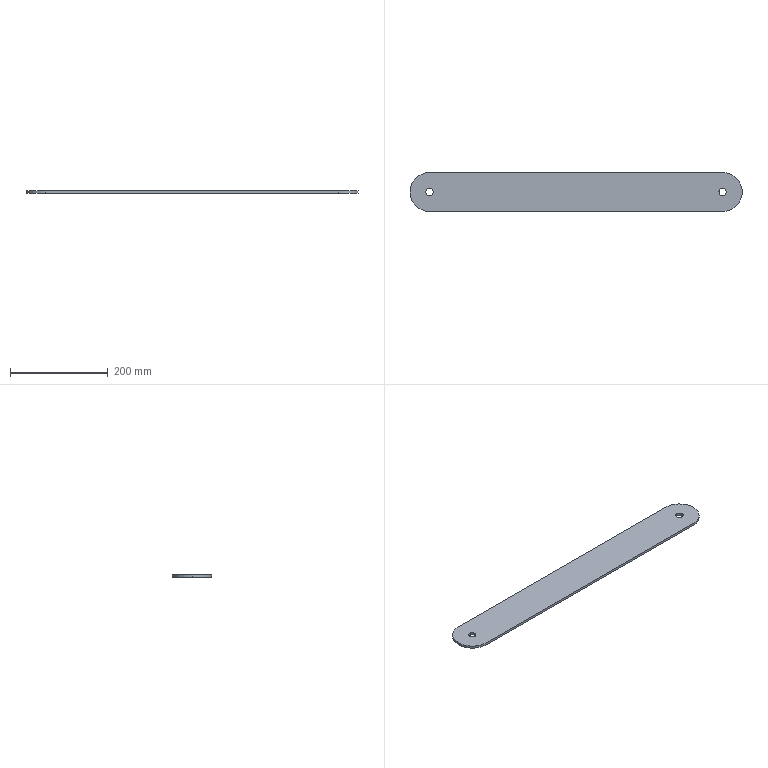Part | SolidWorks | features Extrusion 1, ICE 1 | 1 solid | 11 faces | box 680 x 80 x 5 mm | volume 263366 mm3 | cylinder 7 | plane 4 | commonest cylinder face diameters 15 x4 80 x3
STEP:
#1=CARTESIAN_POINT('',(-7.5,0.,0.));
#2=VERTEX_POINT('',#1);
#3=CARTESIAN_POINT('',(7.5,0.,0.));
#4=VERTEX_POINT('',#3);
#5=CARTESIAN_POINT('',(0.,0.,0.));
#6=DIRECTION('',(0.,0.,1.));
#7=DIRECTION('',(1.,0.,0.));
#8=AXIS2_PLACEMENT_3D('',#5,#6,#7);
#9=CIRCLE('',#8,7.5);
#10=EDGE_CURVE('',#2,#4,#9,.T.);
#11=ORIENTED_EDGE('',*,*,#10,.F.);
#12=CARTESIAN_POINT('',(-7.5,0.,5.));
#13=VERTEX_POINT('',#12);
#14=CARTESIAN_POINT('',(-7.5,0.,0.));
#15=DIRECTION('',(0.,0.,1.));
#16=VECTOR('',#15,1000.);
#17=LINE('',#14,#16);
#18=EDGE_CURVE('',#2,#13,#17,.T.);
#19=ORIENTED_EDGE('',*,*,#18,.T.);
#20=CARTESIAN_POINT('',(7.5,0.,5.));
#21=VERTEX_POINT('',#20);
#22=CARTESIAN_POINT('',(0.,0.,5.));
#23=DIRECTION('',(0.,0.,1.));
#24=DIRECTION('',(1.,0.,0.));
#25=AXIS2_PLACEMENT_3D('',#22,#23,#24);
#26=CIRCLE('',#25,7.5);
#27=EDGE_CURVE('',#13,#21,#26,.T.);
#28=ORIENTED_EDGE('',*,*,#27,.T.);
#29=CARTESIAN_POINT('',(7.5,0.,0.));
#30=DIRECTION('',(0.,0.,1.));
#31=VECTOR('',#30,1000.);
#32=LINE('',#29,#31);
#33=EDGE_CURVE('',#4,#21,#32,.T.);
#34=ORIENTED_EDGE('',*,*,#33,.F.);
#35=EDGE_LOOP('',(#11,#19,#28,#34));
#36=FACE_OUTER_BOUND('',#35,.T.);
#37=CARTESIAN_POINT('',(0.,0.,0.));
#38=DIRECTION('',(0.,0.,1.));
#39=DIRECTION('',(1.,0.,0.));
#40=AXIS2_PLACEMENT_3D('',#37,#38,#39);
#41=CYLINDRICAL_SURFACE('',#40,7.5);
#42=ADVANCED_FACE('',(#36),#41,.F.);
#43=CARTESIAN_POINT('',(592.5,0.,0.));
#44=VERTEX_POINT('',#43);
#45=CARTESIAN_POINT('',(607.5,0.,0.));
#46=VERTEX_POINT('',#45);
#47=CARTESIAN_POINT('',(600.,0.,0.));
#48=DIRECTION('',(0.,0.,1.));
#49=DIRECTION('',(1.,0.,0.));
#50=AXIS2_PLACEMENT_3D('',#47,#48,#49);
#51=CIRCLE('',#50,7.5);
#52=EDGE_CURVE('',#44,#46,#51,.T.);
#53=ORIENTED_EDGE('',*,*,#52,.F.);
#54=CARTESIAN_POINT('',(592.5,0.,5.));
#55=VERTEX_POINT('',#54);
#56=CARTESIAN_POINT('',(592.5,0.,0.));
#57=DIRECTION('',(0.,0.,1.));
#58=VECTOR('',#57,1000.);
#59=LINE('',#56,#58);
#60=EDGE_CURVE('',#44,#55,#59,.T.);
#61=ORIENTED_EDGE('',*,*,#60,.T.);
#62=CARTESIAN_POINT('',(607.5,0.,5.));
#63=VERTEX_POINT('',#62);
#64=CARTESIAN_POINT('',(600.,0.,5.));
#65=DIRECTION('',(0.,0.,1.));
#66=DIRECTION('',(1.,0.,0.));
#67=AXIS2_PLACEMENT_3D('',#64,#65,#66);
#68=CIRCLE('',#67,7.5);
#69=EDGE_CURVE('',#55,#63,#68,.T.);
#70=ORIENTED_EDGE('',*,*,#69,.T.);
#71=CARTESIAN_POINT('',(607.5,0.,0.));
#72=DIRECTION('',(0.,0.,1.));
#73=VECTOR('',#72,1000.);
#74=LINE('',#71,#73);
#75=EDGE_CURVE('',#46,#63,#74,.T.);
#76=ORIENTED_EDGE('',*,*,#75,.F.);
#77=EDGE_LOOP('',(#53,#61,#70,#76));
#78=FACE_OUTER_BOUND('',#77,.T.);
#79=CARTESIAN_POINT('',(600.,0.,0.));
#80=DIRECTION('',(0.,0.,1.));
#81=DIRECTION('',(1.,0.,0.));
#82=AXIS2_PLACEMENT_3D('',#79,#80,#81);
#83=CYLINDRICAL_SURFACE('',#82,7.5);
#84=ADVANCED_FACE('',(#78),#83,.F.);
#85=CARTESIAN_POINT('',(-40.,0.,5.));
#86=VERTEX_POINT('',#85);
#87=CARTESIAN_POINT('',(0.,-40.,5.));
#88=VERTEX_POINT('',#87);
#89=CARTESIAN_POINT('',(0.,0.,5.));
#90=DIRECTION('',(0.,0.,1.));
#91=DIRECTION('',(1.,0.,0.));
#92=AXIS2_PLACEMENT_3D('',#89,#90,#91);
#93=CIRCLE('',#92,40.);
#94=EDGE_CURVE('',#86,#88,#93,.T.);
#95=ORIENTED_EDGE('',*,*,#94,.F.);
#96=CARTESIAN_POINT('',(-40.,0.,0.));
#97=VERTEX_POINT('',#96);
#98=CARTESIAN_POINT('',(-40.,0.,5.));
#99=DIRECTION('',(0.,0.,-1.));
#100=VECTOR('',#99,1000.);
#101=LINE('',#98,#100);
#102=EDGE_CURVE('',#86,#97,#101,.T.);
#103=ORIENTED_EDGE('',*,*,#102,.T.);
#104=CARTESIAN_POINT('',(0.,-40.,0.));
#105=VERTEX_POINT('',#104);
#106=CARTESIAN_POINT('',(0.,0.,0.));
#107=DIRECTION('',(0.,0.,1.));
#108=DIRECTION('',(1.,0.,0.));
#109=AXIS2_PLACEMENT_3D('',#106,#107,#108);
#110=CIRCLE('',#109,40.);
#111=EDGE_CURVE('',#97,#105,#110,.T.);
#112=ORIENTED_EDGE('',*,*,#111,.T.);
#113=CARTESIAN_POINT('',(0.,-40.,5.));
#114=DIRECTION('',(0.,0.,-1.));
#115=VECTOR('',#114,1000.);
#116=LINE('',#113,#115);
#117=EDGE_CURVE('',#88,#105,#116,.T.);
#118=ORIENTED_EDGE('',*,*,#117,.F.);
#119=EDGE_LOOP('',(#95,#103,#112,#118));
#120=FACE_OUTER_BOUND('',#119,.T.);
#121=CARTESIAN_POINT('',(0.,0.,5.));
#122=DIRECTION('',(0.,0.,-1.));
#123=DIRECTION('',(-1.,0.,0.));
#124=AXIS2_PLACEMENT_3D('',#121,#122,#123);
#125=CYLINDRICAL_SURFACE('',#124,40.);
#126=ADVANCED_FACE('',(#120),#125,.T.);
#127=ORIENTED_EDGE('',*,*,#102,.F.);
#128=CARTESIAN_POINT('',(0.,40.,5.));
#129=VERTEX_POINT('',#128);
#130=CARTESIAN_POINT('',(0.,0.,5.));
#131=DIRECTION('',(0.,0.,1.));
#132=DIRECTION('',(1.,0.,0.));
#133=AXIS2_PLACEMENT_3D('',#130,#131,#132);
#134=CIRCLE('',#133,40.);
#135=EDGE_CURVE('',#129,#86,#134,.T.);
#136=ORIENTED_EDGE('',*,*,#135,.F.);
#137=CARTESIAN_POINT('',(0.,40.,0.));
#138=VERTEX_POINT('',#137);
#139=CARTESIAN_POINT('',(0.,40.,5.));
#140=DIRECTION('',(0.,0.,-1.));
#141=VECTOR('',#140,1000.);
#142=LINE('',#139,#141);
#143=EDGE_CURVE('',#129,#138,#142,.T.);
#144=ORIENTED_EDGE('',*,*,#143,.T.);
#145=CARTESIAN_POINT('',(0.,0.,0.));
#146=DIRECTION('',(0.,0.,1.));
#147=DIRECTION('',(1.,0.,0.));
#148=AXIS2_PLACEMENT_3D('',#145,#146,#147);
#149=CIRCLE('',#148,40.);
#150=EDGE_CURVE('',#138,#97,#149,.T.);
#151=ORIENTED_EDGE('',*,*,#150,.T.);
#152=EDGE_LOOP('',(#127,#136,#144,#151));
#153=FACE_OUTER_BOUND('',#152,.T.);
#154=CARTESIAN_POINT('',(0.,0.,5.));
#155=DIRECTION('',(0.,0.,-1.));
#156=DIRECTION('',(-1.,0.,0.));
#157=AXIS2_PLACEMENT_3D('',#154,#155,#156);
#158=CYLINDRICAL_SURFACE('',#157,40.);
#159=ADVANCED_FACE('',(#153),#158,.T.);
#160=CARTESIAN_POINT('',(600.,-40.,0.));
#161=VERTEX_POINT('',#160);
#162=CARTESIAN_POINT('',(0.,-40.,0.));
#163=DIRECTION('',(1.,0.,0.));
#164=VECTOR('',#163,1000.);
#165=LINE('',#162,#164);
#166=EDGE_CURVE('',#105,#161,#165,.T.);
#167=ORIENTED_EDGE('',*,*,#166,.T.);
#168=CARTESIAN_POINT('',(600.,-40.,5.));
#169=VERTEX_POINT('',#168);
#170=CARTESIAN_POINT('',(600.,-40.,5.));
#171=DIRECTION('',(0.,0.,-1.));
#172=VECTOR('',#171,1000.);
#173=LINE('',#170,#172);
#174=EDGE_CURVE('',#169,#161,#173,.T.);
#175=ORIENTED_EDGE('',*,*,#174,.F.);
#176=CARTESIAN_POINT('',(0.,-40.,5.));
#177=DIRECTION('',(1.,0.,0.));
#178=VECTOR('',#177,1000.);
#179=LINE('',#176,#178);
#180=EDGE_CURVE('',#88,#169,#179,.T.);
#181=ORIENTED_EDGE('',*,*,#180,.F.);
#182=ORIENTED_EDGE('',*,*,#117,.T.);
#183=EDGE_LOOP('',(#167,#175,#181,#182));
#184=FACE_OUTER_BOUND('',#183,.T.);
#185=CARTESIAN_POINT('',(0.,-40.,5.));
#186=DIRECTION('',(0.,1.,0.));
#187=DIRECTION('',(0.,0.,1.));
#188=AXIS2_PLACEMENT_3D('',#185,#186,#187);
#189=PLANE('',#188);
#190=ADVANCED_FACE('',(#184),#189,.F.);
#191=CARTESIAN_POINT('',(600.,40.,0.));
#192=VERTEX_POINT('',#191);
#193=CARTESIAN_POINT('',(600.,0.,0.));
#194=DIRECTION('',(0.,0.,1.));
#195=DIRECTION('',(1.,0.,0.));
#196=AXIS2_PLACEMENT_3D('',#193,#194,#195);
#197=CIRCLE('',#196,40.);
#198=EDGE_CURVE('',#161,#192,#197,.T.);
#199=ORIENTED_EDGE('',*,*,#198,.T.);
#200=CARTESIAN_POINT('',(600.,40.,5.));
#201=VERTEX_POINT('',#200);
#202=CARTESIAN_POINT('',(600.,40.,5.));
#203=DIRECTION('',(0.,0.,-1.));
#204=VECTOR('',#203,1000.);
#205=LINE('',#202,#204);
#206=EDGE_CURVE('',#201,#192,#205,.T.);
#207=ORIENTED_EDGE('',*,*,#206,.F.);
#208=CARTESIAN_POINT('',(600.,0.,5.));
#209=DIRECTION('',(0.,0.,1.));
#210=DIRECTION('',(1.,0.,0.));
#211=AXIS2_PLACEMENT_3D('',#208,#209,#210);
#212=CIRCLE('',#211,40.);
#213=EDGE_CURVE('',#169,#201,#212,.T.);
#214=ORIENTED_EDGE('',*,*,#213,.F.);
#215=ORIENTED_EDGE('',*,*,#174,.T.);
#216=EDGE_LOOP('',(#199,#207,#214,#215));
#217=FACE_OUTER_BOUND('',#216,.T.);
#218=CARTESIAN_POINT('',(600.,0.,5.));
#219=DIRECTION('',(0.,0.,-1.));
#220=DIRECTION('',(-1.,0.,0.));
#221=AXIS2_PLACEMENT_3D('',#218,#219,#220);
#222=CYLINDRICAL_SURFACE('',#221,40.);
#223=ADVANCED_FACE('',(#217),#222,.T.);
#224=CARTESIAN_POINT('',(0.,40.,0.));
#225=DIRECTION('',(-1.,0.,0.));
#226=VECTOR('',#225,1000.);
#227=LINE('',#224,#226);
#228=EDGE_CURVE('',#192,#138,#227,.T.);
#229=ORIENTED_EDGE('',*,*,#228,.T.);
#230=ORIENTED_EDGE('',*,*,#143,.F.);
#231=CARTESIAN_POINT('',(0.,40.,5.));
#232=DIRECTION('',(-1.,0.,0.));
#233=VECTOR('',#232,1000.);
#234=LINE('',#231,#233);
#235=EDGE_CURVE('',#201,#129,#234,.T.);
#236=ORIENTED_EDGE('',*,*,#235,.F.);
#237=ORIENTED_EDGE('',*,*,#206,.T.);
#238=EDGE_LOOP('',(#229,#230,#236,#237));
#239=FACE_OUTER_BOUND('',#238,.T.);
#240=CARTESIAN_POINT('',(0.,40.,5.));
#241=DIRECTION('',(0.,-1.,0.));
#242=DIRECTION('',(0.,0.,-1.));
#243=AXIS2_PLACEMENT_3D('',#240,#241,#242);
#244=PLANE('',#243);
#245=ADVANCED_FACE('',(#239),#244,.F.);
#246=CARTESIAN_POINT('',(0.,0.,5.));
#247=DIRECTION('',(0.,0.,1.));
#248=DIRECTION('',(1.,0.,0.));
#249=AXIS2_PLACEMENT_3D('',#246,#247,#248);
#250=CIRCLE('',#249,7.5);
#251=EDGE_CURVE('',#21,#13,#250,.T.);
#252=ORIENTED_EDGE('',*,*,#251,.F.);
#253=ORIENTED_EDGE('',*,*,#27,.F.);
#254=EDGE_LOOP('',(#252,#253));
#255=FACE_BOUND('',#254,.T.);
#256=CARTESIAN_POINT('',(600.,0.,5.));
#257=DIRECTION('',(0.,0.,1.));
#258=DIRECTION('',(1.,0.,0.));
#259=AXIS2_PLACEMENT_3D('',#256,#257,#258);
#260=CIRCLE('',#259,7.5);
#261=EDGE_CURVE('',#63,#55,#260,.T.);
#262=ORIENTED_EDGE('',*,*,#261,.F.);
#263=ORIENTED_EDGE('',*,*,#69,.F.);
#264=EDGE_LOOP('',(#262,#263));
#265=FACE_BOUND('',#264,.T.);
#266=ORIENTED_EDGE('',*,*,#135,.T.);
#267=ORIENTED_EDGE('',*,*,#94,.T.);
#268=ORIENTED_EDGE('',*,*,#180,.T.);
#269=ORIENTED_EDGE('',*,*,#213,.T.);
#270=ORIENTED_EDGE('',*,*,#235,.T.);
#271=EDGE_LOOP('',(#266,#267,#268,#269,#270));
#272=FACE_OUTER_BOUND('',#271,.T.);
#273=CARTESIAN_POINT('',(0.,0.,5.));
#274=DIRECTION('',(0.,0.,1.));
#275=DIRECTION('',(1.,0.,0.));
#276=AXIS2_PLACEMENT_3D('',#273,#274,#275);
#277=PLANE('',#276);
#278=ADVANCED_FACE('',(#255,#265,#272),#277,.T.);
#279=CARTESIAN_POINT('',(0.,0.,0.));
#280=DIRECTION('',(0.,0.,1.));
#281=DIRECTION('',(1.,0.,0.));
#282=AXIS2_PLACEMENT_3D('',#279,#280,#281);
#283=CIRCLE('',#282,7.5);
#284=EDGE_CURVE('',#4,#2,#283,.T.);
#285=ORIENTED_EDGE('',*,*,#284,.T.);
#286=ORIENTED_EDGE('',*,*,#10,.T.);
#287=EDGE_LOOP('',(#285,#286));
#288=FACE_BOUND('',#287,.T.);
#289=CARTESIAN_POINT('',(600.,0.,0.));
#290=DIRECTION('',(0.,0.,1.));
#291=DIRECTION('',(1.,0.,0.));
#292=AXIS2_PLACEMENT_3D('',#289,#290,#291);
#293=CIRCLE('',#292,7.5);
#294=EDGE_CURVE('',#46,#44,#293,.T.);
#295=ORIENTED_EDGE('',*,*,#294,.T.);
#296=ORIENTED_EDGE('',*,*,#52,.T.);
#297=EDGE_LOOP('',(#295,#296));
#298=FACE_BOUND('',#297,.T.);
#299=ORIENTED_EDGE('',*,*,#150,.F.);
#300=ORIENTED_EDGE('',*,*,#228,.F.);
#301=ORIENTED_EDGE('',*,*,#198,.F.);
#302=ORIENTED_EDGE('',*,*,#166,.F.);
#303=ORIENTED_EDGE('',*,*,#111,.F.);
#304=EDGE_LOOP('',(#299,#300,#301,#302,#303));
#305=FACE_OUTER_BOUND('',#304,.T.);
#306=CARTESIAN_POINT('',(0.,0.,0.));
#307=DIRECTION('',(0.,0.,1.));
#308=DIRECTION('',(1.,0.,0.));
#309=AXIS2_PLACEMENT_3D('',#306,#307,#308);
#310=PLANE('',#309);
#311=ADVANCED_FACE('',(#288,#298,#305),#310,.F.);
#312=ORIENTED_EDGE('',*,*,#60,.F.);
#313=ORIENTED_EDGE('',*,*,#294,.F.);
#314=ORIENTED_EDGE('',*,*,#75,.T.);
#315=ORIENTED_EDGE('',*,*,#261,.T.);
#316=EDGE_LOOP('',(#312,#313,#314,#315));
#317=FACE_OUTER_BOUND('',#316,.T.);
#318=CARTESIAN_POINT('',(600.,0.,0.));
#319=DIRECTION('',(0.,0.,1.));
#320=DIRECTION('',(1.,0.,0.));
#321=AXIS2_PLACEMENT_3D('',#318,#319,#320);
#322=CYLINDRICAL_SURFACE('',#321,7.5);
#323=ADVANCED_FACE('',(#317),#322,.F.);
#324=ORIENTED_EDGE('',*,*,#18,.F.);
#325=ORIENTED_EDGE('',*,*,#284,.F.);
#326=ORIENTED_EDGE('',*,*,#33,.T.);
#327=ORIENTED_EDGE('',*,*,#251,.T.);
#328=EDGE_LOOP('',(#324,#325,#326,#327));
#329=FACE_OUTER_BOUND('',#328,.T.);
#330=CARTESIAN_POINT('',(0.,0.,0.));
#331=DIRECTION('',(0.,0.,1.));
#332=DIRECTION('',(1.,0.,0.));
#333=AXIS2_PLACEMENT_3D('',#330,#331,#332);
#334=CYLINDRICAL_SURFACE('',#333,7.5);
#335=ADVANCED_FACE('',(#329),#334,.F.);
#336=CLOSED_SHELL('',(#42,#84,#126,#159,#190,#223,#245,#278,#311,#323,#335));
#337=MANIFOLD_SOLID_BREP('',#336);
#338=CARTESIAN_POINT('',(0.,0.,0.));
#339=DIRECTION('',(0.,0.,1.));
#340=DIRECTION('',(1.,0.,0.));
#341=AXIS2_PLACEMENT_3D('',#338,#339,#340);
#342=(LENGTH_UNIT()NAMED_UNIT(*)SI_UNIT(.MILLI.,.METRE.));
#343=UNCERTAINTY_MEASURE_WITH_UNIT(LENGTH_MEASURE(0.00001),#342,'','');
#344=(NAMED_UNIT(*)PLANE_ANGLE_UNIT()SI_UNIT($,.RADIAN.));
#345=(NAMED_UNIT(*)SI_UNIT($,.STERADIAN.)SOLID_ANGLE_UNIT());
#346=(GEOMETRIC_REPRESENTATION_CONTEXT(3)GLOBAL_UNCERTAINTY_ASSIGNED_CONTEXT((#343))GLOBAL_UNIT_ASSIGNED_CONTEXT((#342,#344,#345))REPRESENTATION_CONTEXT('',''));
#347=ADVANCED_BREP_SHAPE_REPRESENTATION('',(#337,#341),#346);